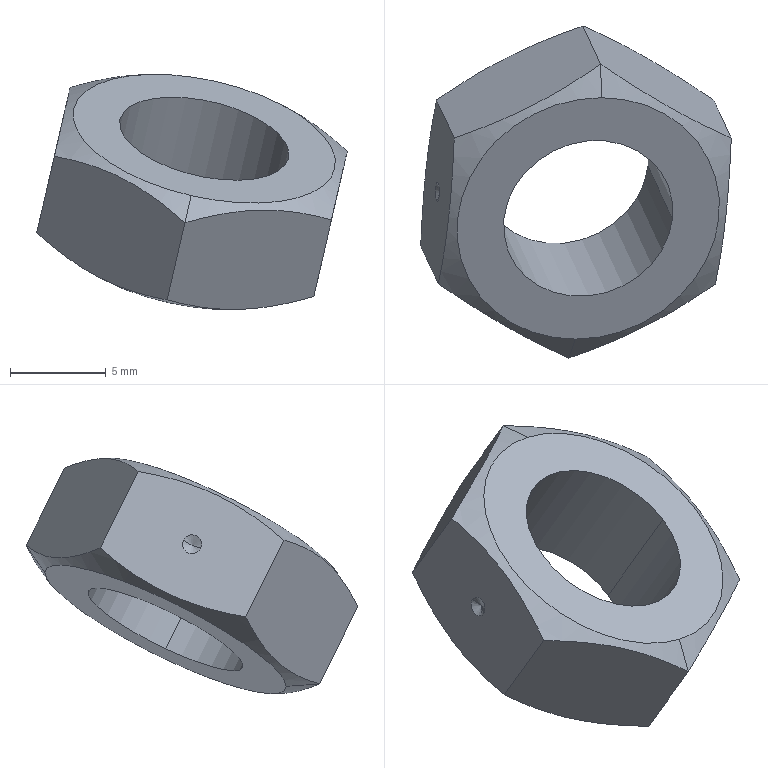Part | SolidWorks | features BaseBody 1 | 1 solid | 18 faces | box 16.219 x 17.338 x 12.294 mm | volume 776.179 mm3 | plane 8 | cone 8 | cylinder 2 | commonest cylinder face diameters 9.035 x2
STEP:
#1=CARTESIAN_POINT('',(1929.341,-170.963,831.295));
#2=VERTEX_POINT('',#1);
#3=CARTESIAN_POINT('',(1930.707,-158.364,837.245));
#4=VERTEX_POINT('',#3);
#5=CARTESIAN_POINT('',(1930.024,-164.664,834.27));
#6=DIRECTION('',(0.2015,-0.436,0.8771));
#7=DIRECTION('',(-0.09761,-0.8999,-0.425));
#8=AXIS2_PLACEMENT_3D('',#5,#6,#7);
#9=CIRCLE('',#8,7.);
#10=EDGE_CURVE('',#2,#4,#9,.T.);
#11=ORIENTED_EDGE('',*,*,#10,.T.);
#12=CARTESIAN_POINT('',(1930.024,-164.664,834.27));
#13=DIRECTION('',(0.2015,-0.436,0.8771));
#14=DIRECTION('',(0.09761,0.8999,0.425));
#15=AXIS2_PLACEMENT_3D('',#12,#13,#14);
#16=CIRCLE('',#15,7.);
#17=EDGE_CURVE('',#4,#2,#16,.T.);
#18=ORIENTED_EDGE('',*,*,#17,.T.);
#19=EDGE_LOOP('',(#11,#18));
#20=FACE_OUTER_BOUND('',#19,.T.);
#21=CARTESIAN_POINT('',(1934.427,-164.664,833.259));
#22=VERTEX_POINT('',#21);
#23=CARTESIAN_POINT('',(1925.621,-164.664,835.281));
#24=VERTEX_POINT('',#23);
#25=CARTESIAN_POINT('',(1930.024,-164.664,834.27));
#26=DIRECTION('',(-0.2015,0.436,-0.8771));
#27=DIRECTION('',(0.9746,0.,-0.2239));
#28=AXIS2_PLACEMENT_3D('',#25,#26,#27);
#29=CIRCLE('',#28,4.517);
#30=EDGE_CURVE('',#22,#24,#29,.T.);
#31=ORIENTED_EDGE('',*,*,#30,.T.);
#32=CARTESIAN_POINT('',(1930.024,-164.664,834.27));
#33=DIRECTION('',(-0.2015,0.436,-0.8771));
#34=DIRECTION('',(-0.9746,0.,0.2239));
#35=AXIS2_PLACEMENT_3D('',#32,#33,#34);
#36=CIRCLE('',#35,4.517);
#37=EDGE_CURVE('',#24,#22,#36,.T.);
#38=ORIENTED_EDGE('',*,*,#37,.T.);
#39=EDGE_LOOP('',(#31,#38));
#40=FACE_BOUND('',#39,.T.);
#41=CARTESIAN_POINT('',(1936.408,-171.215,829.546));
#42=DIRECTION('',(0.2015,-0.436,0.8771));
#43=DIRECTION('',(0.09761,0.8999,0.425));
#44=AXIS2_PLACEMENT_3D('',#41,#42,#43);
#45=PLANE('',#44);
#46=ADVANCED_FACE('',(#20,#40),#45,.T.);
#47=CARTESIAN_POINT('',(1924.342,-161.895,829.712));
#48=VERTEX_POINT('',#47);
#49=CARTESIAN_POINT('',(1925.621,-164.664,835.281));
#50=DIRECTION('',(-0.2015,0.436,-0.8771));
#51=VECTOR('',#50,1000.);
#52=LINE('',#49,#51);
#53=EDGE_CURVE('',#24,#48,#52,.T.);
#54=ORIENTED_EDGE('',*,*,#53,.T.);
#55=CARTESIAN_POINT('',(1933.147,-161.895,827.689));
#56=VERTEX_POINT('',#55);
#57=CARTESIAN_POINT('',(1928.744,-161.895,828.7));
#58=DIRECTION('',(-0.2015,0.436,-0.8771));
#59=DIRECTION('',(-0.9746,0.,0.2239));
#60=AXIS2_PLACEMENT_3D('',#57,#58,#59);
#61=CIRCLE('',#60,4.517);
#62=EDGE_CURVE('',#48,#56,#61,.T.);
#63=ORIENTED_EDGE('',*,*,#62,.T.);
#64=CARTESIAN_POINT('',(1934.427,-164.664,833.259));
#65=DIRECTION('',(0.2015,-0.436,0.8771));
#66=VECTOR('',#65,1000.);
#67=LINE('',#64,#66);
#68=EDGE_CURVE('',#56,#22,#67,.T.);
#69=ORIENTED_EDGE('',*,*,#68,.T.);
#70=ORIENTED_EDGE('',*,*,#37,.F.);
#71=EDGE_LOOP('',(#54,#63,#69,#70));
#72=FACE_OUTER_BOUND('',#71,.T.);
#73=CARTESIAN_POINT('',(1930.049,-164.719,834.381));
#74=DIRECTION('',(-0.2015,0.436,-0.8771));
#75=DIRECTION('',(-0.9746,0.,0.2239));
#76=AXIS2_PLACEMENT_3D('',#73,#74,#75);
#77=CYLINDRICAL_SURFACE('',#76,4.518);
#78=ADVANCED_FACE('',(#72),#77,.F.);
#79=ORIENTED_EDGE('',*,*,#68,.F.);
#80=CARTESIAN_POINT('',(1928.744,-161.895,828.7));
#81=DIRECTION('',(-0.2015,0.436,-0.8771));
#82=DIRECTION('',(0.9746,0.,-0.2239));
#83=AXIS2_PLACEMENT_3D('',#80,#81,#82);
#84=CIRCLE('',#83,4.517);
#85=EDGE_CURVE('',#56,#48,#84,.T.);
#86=ORIENTED_EDGE('',*,*,#85,.T.);
#87=ORIENTED_EDGE('',*,*,#53,.F.);
#88=ORIENTED_EDGE('',*,*,#30,.F.);
#89=EDGE_LOOP('',(#79,#86,#87,#88));
#90=FACE_OUTER_BOUND('',#89,.T.);
#91=CARTESIAN_POINT('',(1930.049,-164.719,834.381));
#92=DIRECTION('',(-0.2015,0.436,-0.8771));
#93=DIRECTION('',(-0.9746,0.,0.2239));
#94=AXIS2_PLACEMENT_3D('',#91,#92,#93);
#95=CYLINDRICAL_SURFACE('',#94,4.518);
#96=ADVANCED_FACE('',(#90),#95,.F.);
#97=CARTESIAN_POINT('',(1928.061,-168.194,825.726));
#98=VERTEX_POINT('',#97);
#99=CARTESIAN_POINT('',(1929.428,-155.595,831.675));
#100=VERTEX_POINT('',#99);
#101=CARTESIAN_POINT('',(1928.744,-161.895,828.7));
#102=DIRECTION('',(0.2015,-0.436,0.8771));
#103=DIRECTION('',(-0.09761,-0.8999,-0.425));
#104=AXIS2_PLACEMENT_3D('',#101,#102,#103);
#105=CIRCLE('',#104,7.);
#106=EDGE_CURVE('',#98,#100,#105,.T.);
#107=ORIENTED_EDGE('',*,*,#106,.F.);
#108=CARTESIAN_POINT('',(1928.744,-161.895,828.7));
#109=DIRECTION('',(0.2015,-0.436,0.8771));
#110=DIRECTION('',(0.09761,0.8999,0.425));
#111=AXIS2_PLACEMENT_3D('',#108,#109,#110);
#112=CIRCLE('',#111,7.);
#113=EDGE_CURVE('',#100,#98,#112,.T.);
#114=ORIENTED_EDGE('',*,*,#113,.F.);
#115=EDGE_LOOP('',(#107,#114));
#116=FACE_OUTER_BOUND('',#115,.T.);
#117=ORIENTED_EDGE('',*,*,#85,.F.);
#118=ORIENTED_EDGE('',*,*,#62,.F.);
#119=EDGE_LOOP('',(#117,#118));
#120=FACE_BOUND('',#119,.T.);
#121=CARTESIAN_POINT('',(1935.129,-168.446,823.977));
#122=DIRECTION('',(-0.2015,0.436,-0.8771));
#123=DIRECTION('',(-0.9746,0.,0.2239));
#124=AXIS2_PLACEMENT_3D('',#121,#122,#123);
#125=PLANE('',#124);
#126=ADVANCED_FACE('',(#116,#120),#125,.T.);
#127=CARTESIAN_POINT('',(1928.09,-169.945,825.849));
#128=VERTEX_POINT('',#127);
#129=CARTESIAN_POINT('',(1928.09,-169.945,825.849));
#130=DIRECTION('',(0.0162,-0.9974,0.07053));
#131=VECTOR('',#130,1000.);
#132=LINE('',#129,#131);
#133=EDGE_CURVE('',#98,#128,#132,.T.);
#134=ORIENTED_EDGE('',*,*,#133,.T.);
#135=CARTESIAN_POINT('',(1921.275,-166.094,829.347));
#136=VERTEX_POINT('',#135);
#137=CARTESIAN_POINT('',(1921.275,-166.094,829.347));
#138=CARTESIAN_POINT('',(1921.79,-166.32,828.884));
#139=CARTESIAN_POINT('',(1922.316,-166.563,828.45));
#140=CARTESIAN_POINT('',(1923.402,-167.102,827.665));
#141=CARTESIAN_POINT('',(1923.961,-167.397,827.315));
#142=CARTESIAN_POINT('',(1924.83,-167.888,826.868));
#143=CARTESIAN_POINT('',(1925.125,-168.06,826.732));
#144=CARTESIAN_POINT('',(1925.713,-168.411,826.49));
#145=CARTESIAN_POINT('',(1926.008,-168.593,826.383));
#146=CARTESIAN_POINT('',(1926.896,-169.151,826.098));
#147=CARTESIAN_POINT('',(1927.491,-169.541,825.957));
#148=CARTESIAN_POINT('',(1928.09,-169.945,825.849));
#149=B_SPLINE_CURVE_WITH_KNOTS('',3,(#137,#138,#139,#140,#141,#142,#143,#144,#145,#146,#147,#148),.UNSPECIFIED.,.F.,.F.,(4,2,2,2,2,4),(0.,0.002165,0.004331,0.005413,0.006496,0.008661),.UNSPECIFIED.);
#150=EDGE_CURVE('',#136,#128,#149,.T.);
#151=ORIENTED_EDGE('',*,*,#150,.F.);
#152=CARTESIAN_POINT('',(1922.101,-158.475,832.945));
#153=VERTEX_POINT('',#152);
#154=CARTESIAN_POINT('',(1922.101,-158.475,832.945));
#155=CARTESIAN_POINT('',(1921.994,-159.011,832.478));
#156=CARTESIAN_POINT('',(1921.893,-159.566,832.039));
#157=CARTESIAN_POINT('',(1921.71,-160.734,831.244));
#158=CARTESIAN_POINT('',(1921.629,-161.347,830.888));
#159=CARTESIAN_POINT('',(1921.523,-162.317,830.429));
#160=CARTESIAN_POINT('',(1921.491,-162.649,830.288));
#161=CARTESIAN_POINT('',(1921.433,-163.319,830.036));
#162=CARTESIAN_POINT('',(1921.407,-163.658,829.923));
#163=CARTESIAN_POINT('',(1921.338,-164.685,829.621));
#164=CARTESIAN_POINT('',(1921.302,-165.384,829.468));
#165=CARTESIAN_POINT('',(1921.275,-166.094,829.347));
#166=B_SPLINE_CURVE_WITH_KNOTS('',3,(#154,#155,#156,#157,#158,#159,#160,#161,#162,#163,#164,#165),.UNSPECIFIED.,.F.,.F.,(4,2,2,2,2,4),(0.,0.002137,0.004273,0.005342,0.00641,0.008546),.UNSPECIFIED.);
#167=EDGE_CURVE('',#153,#136,#166,.T.);
#168=ORIENTED_EDGE('',*,*,#167,.F.);
#169=CARTESIAN_POINT('',(1929.753,-154.61,833.091));
#170=VERTEX_POINT('',#169);
#171=CARTESIAN_POINT('',(1929.753,-154.61,833.091));
#172=CARTESIAN_POINT('',(1929.087,-154.837,832.9));
#173=CARTESIAN_POINT('',(1928.424,-155.082,832.741));
#174=CARTESIAN_POINT('',(1927.105,-155.623,832.514));
#175=CARTESIAN_POINT('',(1926.449,-155.92,832.446));
#176=CARTESIAN_POINT('',(1925.473,-156.413,832.427));
#177=CARTESIAN_POINT('',(1925.15,-156.585,832.434));
#178=CARTESIAN_POINT('',(1924.516,-156.938,832.475));
#179=CARTESIAN_POINT('',(1924.204,-157.12,832.509));
#180=CARTESIAN_POINT('',(1923.282,-157.679,832.644));
#181=CARTESIAN_POINT('',(1922.685,-158.071,832.779));
#182=CARTESIAN_POINT('',(1922.101,-158.475,832.945));
#183=B_SPLINE_CURVE_WITH_KNOTS('',3,(#171,#172,#173,#174,#175,#176,#177,#178,#179,#180,#181,#182),.UNSPECIFIED.,.F.,.F.,(4,2,2,2,2,4),(0.,0.002165,0.00433,0.005413,0.006496,0.008661),.UNSPECIFIED.);
#184=EDGE_CURVE('',#170,#153,#183,.T.);
#185=ORIENTED_EDGE('',*,*,#184,.F.);
#186=CARTESIAN_POINT('',(1929.753,-154.61,833.091));
#187=DIRECTION('',(-0.1853,-0.5614,-0.8066));
#188=VECTOR('',#187,1000.);
#189=LINE('',#186,#188);
#190=EDGE_CURVE('',#170,#100,#189,.T.);
#191=ORIENTED_EDGE('',*,*,#190,.T.);
#192=ORIENTED_EDGE('',*,*,#113,.T.);
#193=EDGE_LOOP('',(#134,#151,#168,#185,#191,#192));
#194=FACE_OUTER_BOUND('',#193,.T.);
#195=CARTESIAN_POINT('',(1928.741,-161.887,828.685));
#196=DIRECTION('',(0.2015,-0.436,0.8771));
#197=DIRECTION('',(-0.09761,-0.8999,-0.425));
#198=AXIS2_PLACEMENT_3D('',#195,#196,#197);
#199=CONICAL_SURFACE('',#198,6.969,1.047);
#200=ADVANCED_FACE('',(#194),#199,.T.);
#201=ORIENTED_EDGE('',*,*,#190,.F.);
#202=CARTESIAN_POINT('',(1936.574,-158.475,829.62));
#203=VERTEX_POINT('',#202);
#204=CARTESIAN_POINT('',(1936.574,-158.475,829.62));
#205=CARTESIAN_POINT('',(1935.977,-158.071,829.726));
#206=CARTESIAN_POINT('',(1935.382,-157.68,829.864));
#207=CARTESIAN_POINT('',(1934.202,-156.937,830.237));
#208=CARTESIAN_POINT('',(1933.617,-156.585,830.473));
#209=CARTESIAN_POINT('',(1932.746,-156.091,830.914));
#210=CARTESIAN_POINT('',(1932.458,-155.933,831.076));
#211=CARTESIAN_POINT('',(1931.894,-155.633,831.423));
#212=CARTESIAN_POINT('',(1931.617,-155.49,831.608));
#213=CARTESIAN_POINT('',(1930.798,-155.083,832.195));
#214=CARTESIAN_POINT('',(1930.27,-154.837,832.628));
#215=CARTESIAN_POINT('',(1929.753,-154.61,833.091));
#216=B_SPLINE_CURVE_WITH_KNOTS('',3,(#204,#205,#206,#207,#208,#209,#210,#211,#212,#213,#214,#215),.UNSPECIFIED.,.F.,.F.,(4,2,2,2,2,4),(0.,0.002165,0.004331,0.005413,0.006496,0.008661),.UNSPECIFIED.);
#217=EDGE_CURVE('',#203,#170,#216,.T.);
#218=ORIENTED_EDGE('',*,*,#217,.F.);
#219=CARTESIAN_POINT('',(1935.748,-166.094,826.023));
#220=VERTEX_POINT('',#219);
#221=CARTESIAN_POINT('',(1935.748,-166.094,826.023));
#222=CARTESIAN_POINT('',(1935.775,-165.385,826.143));
#223=CARTESIAN_POINT('',(1935.811,-164.688,826.296));
#224=CARTESIAN_POINT('',(1935.903,-163.324,826.697));
#225=CARTESIAN_POINT('',(1935.959,-162.657,826.944));
#226=CARTESIAN_POINT('',(1936.065,-161.686,827.402));
#227=CARTESIAN_POINT('',(1936.103,-161.367,827.569));
#228=CARTESIAN_POINT('',(1936.185,-160.749,827.925));
#229=CARTESIAN_POINT('',(1936.228,-160.449,828.114));
#230=CARTESIAN_POINT('',(1936.366,-159.569,828.713));
#231=CARTESIAN_POINT('',(1936.467,-159.011,829.152));
#232=CARTESIAN_POINT('',(1936.574,-158.475,829.62));
#233=B_SPLINE_CURVE_WITH_KNOTS('',3,(#221,#222,#223,#224,#225,#226,#227,#228,#229,#230,#231,#232),.UNSPECIFIED.,.F.,.F.,(4,2,2,2,2,4),(0.,0.002137,0.004273,0.005342,0.00641,0.008546),.UNSPECIFIED.);
#234=EDGE_CURVE('',#220,#203,#233,.T.);
#235=ORIENTED_EDGE('',*,*,#234,.F.);
#236=CARTESIAN_POINT('',(1928.09,-169.945,825.849));
#237=CARTESIAN_POINT('',(1928.674,-169.542,825.685));
#238=CARTESIAN_POINT('',(1929.27,-169.152,825.552));
#239=CARTESIAN_POINT('',(1930.497,-168.411,825.378));
#240=CARTESIAN_POINT('',(1931.127,-168.059,825.336));
#241=CARTESIAN_POINT('',(1932.104,-167.568,825.358));
#242=CARTESIAN_POINT('',(1932.434,-167.41,825.38));
#243=CARTESIAN_POINT('',(1933.093,-167.112,825.448));
#244=CARTESIAN_POINT('',(1933.424,-166.97,825.495));
#245=CARTESIAN_POINT('',(1934.417,-166.564,825.669));
#246=CARTESIAN_POINT('',(1935.081,-166.32,825.831));
#247=CARTESIAN_POINT('',(1935.748,-166.094,826.023));
#248=B_SPLINE_CURVE_WITH_KNOTS('',3,(#236,#237,#238,#239,#240,#241,#242,#243,#244,#245,#246,#247),.UNSPECIFIED.,.F.,.F.,(4,2,2,2,2,4),(0.,0.002165,0.00433,0.005413,0.006496,0.008661),.UNSPECIFIED.);
#249=EDGE_CURVE('',#128,#220,#248,.T.);
#250=ORIENTED_EDGE('',*,*,#249,.F.);
#251=ORIENTED_EDGE('',*,*,#133,.F.);
#252=ORIENTED_EDGE('',*,*,#106,.T.);
#253=EDGE_LOOP('',(#201,#218,#235,#250,#251,#252));
#254=FACE_OUTER_BOUND('',#253,.T.);
#255=CARTESIAN_POINT('',(1928.741,-161.887,828.685));
#256=DIRECTION('',(0.2015,-0.436,0.8771));
#257=DIRECTION('',(-0.09761,-0.8999,-0.425));
#258=AXIS2_PLACEMENT_3D('',#255,#256,#257);
#259=CONICAL_SURFACE('',#258,6.969,1.047);
#260=ADVANCED_FACE('',(#254),#259,.T.);
#261=CARTESIAN_POINT('',(1936.667,-168.084,830.025));
#262=VERTEX_POINT('',#261);
#263=CARTESIAN_POINT('',(1936.667,-168.084,830.025));
#264=DIRECTION('',(-0.2015,0.436,-0.8771));
#265=VECTOR('',#264,1000.);
#266=LINE('',#263,#265);
#267=EDGE_CURVE('',#262,#220,#266,.T.);
#268=ORIENTED_EDGE('',*,*,#267,.F.);
#269=CARTESIAN_POINT('',(1929.015,-171.948,829.88));
#270=VERTEX_POINT('',#269);
#271=CARTESIAN_POINT('',(1929.015,-171.948,829.88));
#272=CARTESIAN_POINT('',(1929.681,-171.721,830.07));
#273=CARTESIAN_POINT('',(1930.344,-171.477,830.229));
#274=CARTESIAN_POINT('',(1931.663,-170.935,830.457));
#275=CARTESIAN_POINT('',(1932.319,-170.638,830.525));
#276=CARTESIAN_POINT('',(1933.295,-170.145,830.543));
#277=CARTESIAN_POINT('',(1933.619,-169.974,830.536));
#278=CARTESIAN_POINT('',(1934.253,-169.621,830.495));
#279=CARTESIAN_POINT('',(1934.564,-169.439,830.461));
#280=CARTESIAN_POINT('',(1935.486,-168.879,830.326));
#281=CARTESIAN_POINT('',(1936.083,-168.488,830.191));
#282=CARTESIAN_POINT('',(1936.667,-168.084,830.025));
#283=B_SPLINE_CURVE_WITH_KNOTS('',3,(#271,#272,#273,#274,#275,#276,#277,#278,#279,#280,#281,#282),.UNSPECIFIED.,.F.,.F.,(4,2,2,2,2,4),(0.,0.002165,0.00433,0.005413,0.006496,0.008661),.UNSPECIFIED.);
#284=EDGE_CURVE('',#270,#262,#283,.T.);
#285=ORIENTED_EDGE('',*,*,#284,.F.);
#286=CARTESIAN_POINT('',(1929.015,-171.948,829.88));
#287=DIRECTION('',(-0.2015,0.436,-0.8771));
#288=VECTOR('',#287,1000.);
#289=LINE('',#286,#288);
#290=EDGE_CURVE('',#270,#128,#289,.T.);
#291=ORIENTED_EDGE('',*,*,#290,.T.);
#292=ORIENTED_EDGE('',*,*,#249,.T.);
#293=EDGE_LOOP('',(#268,#285,#291,#292));
#294=FACE_OUTER_BOUND('',#293,.T.);
#295=CARTESIAN_POINT('',(1936.98,-168.352,830.724));
#296=DIRECTION('',(0.4028,-0.7794,-0.48));
#297=DIRECTION('',(-0.8929,-0.45,-0.0186));
#298=AXIS2_PLACEMENT_3D('',#295,#296,#297);
#299=PLANE('',#298);
#300=ADVANCED_FACE('',(#294),#299,.T.);
#301=ORIENTED_EDGE('',*,*,#290,.F.);
#302=CARTESIAN_POINT('',(1922.194,-168.084,833.35));
#303=VERTEX_POINT('',#302);
#304=CARTESIAN_POINT('',(1922.194,-168.084,833.35));
#305=CARTESIAN_POINT('',(1922.791,-168.487,833.244));
#306=CARTESIAN_POINT('',(1923.386,-168.878,833.106));
#307=CARTESIAN_POINT('',(1924.566,-169.621,832.733));
#308=CARTESIAN_POINT('',(1925.152,-169.974,832.498));
#309=CARTESIAN_POINT('',(1926.022,-170.467,832.056));
#310=CARTESIAN_POINT('',(1926.31,-170.626,831.894));
#311=CARTESIAN_POINT('',(1926.875,-170.926,831.548));
#312=CARTESIAN_POINT('',(1927.152,-171.068,831.362));
#313=CARTESIAN_POINT('',(1927.97,-171.476,830.775));
#314=CARTESIAN_POINT('',(1928.499,-171.721,830.342));
#315=CARTESIAN_POINT('',(1929.015,-171.948,829.88));
#316=B_SPLINE_CURVE_WITH_KNOTS('',3,(#304,#305,#306,#307,#308,#309,#310,#311,#312,#313,#314,#315),.UNSPECIFIED.,.F.,.F.,(4,2,2,2,2,4),(0.,0.002165,0.004331,0.005413,0.006496,0.008661),.UNSPECIFIED.);
#317=EDGE_CURVE('',#303,#270,#316,.T.);
#318=ORIENTED_EDGE('',*,*,#317,.F.);
#319=CARTESIAN_POINT('',(1922.194,-168.084,833.35));
#320=DIRECTION('',(-0.2015,0.436,-0.8771));
#321=VECTOR('',#320,1000.);
#322=LINE('',#319,#321);
#323=EDGE_CURVE('',#303,#136,#322,.T.);
#324=ORIENTED_EDGE('',*,*,#323,.T.);
#325=ORIENTED_EDGE('',*,*,#150,.T.);
#326=EDGE_LOOP('',(#301,#318,#324,#325));
#327=FACE_OUTER_BOUND('',#326,.T.);
#328=CARTESIAN_POINT('',(1929.308,-172.364,830.492));
#329=DIRECTION('',(-0.5718,-0.7794,-0.2561));
#330=DIRECTION('',(-0.7952,0.45,0.4064));
#331=AXIS2_PLACEMENT_3D('',#328,#329,#330);
#332=PLANE('',#331);
#333=ADVANCED_FACE('',(#327),#332,.T.);
#334=ORIENTED_EDGE('',*,*,#323,.F.);
#335=CARTESIAN_POINT('',(1923.02,-160.465,836.948));
#336=VERTEX_POINT('',#335);
#337=CARTESIAN_POINT('',(1923.02,-160.465,836.948));
#338=CARTESIAN_POINT('',(1922.993,-161.173,836.827));
#339=CARTESIAN_POINT('',(1922.958,-161.871,836.674));
#340=CARTESIAN_POINT('',(1922.866,-163.235,836.274));
#341=CARTESIAN_POINT('',(1922.809,-163.901,836.026));
#342=CARTESIAN_POINT('',(1922.704,-164.872,835.568));
#343=CARTESIAN_POINT('',(1922.665,-165.191,835.401));
#344=CARTESIAN_POINT('',(1922.584,-165.809,835.046));
#345=CARTESIAN_POINT('',(1922.54,-166.11,834.856));
#346=CARTESIAN_POINT('',(1922.403,-166.99,834.257));
#347=CARTESIAN_POINT('',(1922.302,-167.547,833.818));
#348=CARTESIAN_POINT('',(1922.194,-168.084,833.35));
#349=B_SPLINE_CURVE_WITH_KNOTS('',3,(#337,#338,#339,#340,#341,#342,#343,#344,#345,#346,#347,#348),.UNSPECIFIED.,.F.,.F.,(4,2,2,2,2,4),(0.,0.002137,0.004273,0.005342,0.00641,0.008546),.UNSPECIFIED.);
#350=EDGE_CURVE('',#336,#303,#349,.T.);
#351=ORIENTED_EDGE('',*,*,#350,.F.);
#352=CARTESIAN_POINT('',(1923.02,-160.465,836.948));
#353=DIRECTION('',(-0.2015,0.436,-0.8771));
#354=VECTOR('',#353,1000.);
#355=LINE('',#352,#354);
#356=EDGE_CURVE('',#336,#153,#355,.T.);
#357=ORIENTED_EDGE('',*,*,#356,.T.);
#358=ORIENTED_EDGE('',*,*,#167,.T.);
#359=EDGE_LOOP('',(#334,#351,#357,#358));
#360=FACE_OUTER_BOUND('',#359,.T.);
#361=CARTESIAN_POINT('',(1922.196,-162.829,833.36));
#362=VERTEX_POINT('',#361);
#363=CARTESIAN_POINT('',(1922.099,-163.729,832.935));
#364=VERTEX_POINT('',#363);
#365=CARTESIAN_POINT('',(1922.148,-163.279,833.147));
#366=DIRECTION('',(-0.9746,0.,0.2239));
#367=DIRECTION('',(0.09761,0.8999,0.425));
#368=AXIS2_PLACEMENT_3D('',#365,#366,#367);
#369=CIRCLE('',#368,0.5);
#370=EDGE_CURVE('',#362,#364,#369,.T.);
#371=ORIENTED_EDGE('',*,*,#370,.F.);
#372=CARTESIAN_POINT('',(1922.148,-163.279,833.147));
#373=DIRECTION('',(-0.9746,0.,0.2239));
#374=DIRECTION('',(-0.09761,-0.8999,-0.425));
#375=AXIS2_PLACEMENT_3D('',#372,#373,#374);
#376=CIRCLE('',#375,0.5);
#377=EDGE_CURVE('',#364,#362,#376,.T.);
#378=ORIENTED_EDGE('',*,*,#377,.F.);
#379=EDGE_LOOP('',(#371,#378));
#380=FACE_BOUND('',#379,.T.);
#381=CARTESIAN_POINT('',(1922.332,-168.57,833.949));
#382=DIRECTION('',(-0.9746,0.,0.2239));
#383=DIRECTION('',(0.09761,0.8999,0.425));
#384=AXIS2_PLACEMENT_3D('',#381,#382,#383);
#385=PLANE('',#384);
#386=ADVANCED_FACE('',(#360,#380),#385,.T.);
#387=ORIENTED_EDGE('',*,*,#356,.F.);
#388=CARTESIAN_POINT('',(1930.679,-156.613,837.121));
#389=VERTEX_POINT('',#388);
#390=CARTESIAN_POINT('',(1930.679,-156.613,837.121));
#391=CARTESIAN_POINT('',(1930.094,-157.017,837.285));
#392=CARTESIAN_POINT('',(1929.498,-157.406,837.418));
#393=CARTESIAN_POINT('',(1928.272,-158.148,837.592));
#394=CARTESIAN_POINT('',(1927.641,-158.499,837.634));
#395=CARTESIAN_POINT('',(1926.664,-158.991,837.612));
#396=CARTESIAN_POINT('',(1926.334,-159.148,837.591));
#397=CARTESIAN_POINT('',(1925.675,-159.447,837.522));
#398=CARTESIAN_POINT('',(1925.345,-159.589,837.476));
#399=CARTESIAN_POINT('',(1924.352,-159.994,837.301));
#400=CARTESIAN_POINT('',(1923.687,-160.238,837.14));
#401=CARTESIAN_POINT('',(1923.02,-160.465,836.948));
#402=B_SPLINE_CURVE_WITH_KNOTS('',3,(#390,#391,#392,#393,#394,#395,#396,#397,#398,#399,#400,#401),.UNSPECIFIED.,.F.,.F.,(4,2,2,2,2,4),(0.,0.002165,0.00433,0.005413,0.006496,0.008661),.UNSPECIFIED.);
#403=EDGE_CURVE('',#389,#336,#402,.T.);
#404=ORIENTED_EDGE('',*,*,#403,.F.);
#405=CARTESIAN_POINT('',(1930.679,-156.613,837.121));
#406=DIRECTION('',(-0.2015,0.436,-0.8771));
#407=VECTOR('',#406,1000.);
#408=LINE('',#405,#407);
#409=EDGE_CURVE('',#389,#170,#408,.T.);
#410=ORIENTED_EDGE('',*,*,#409,.T.);
#411=ORIENTED_EDGE('',*,*,#184,.T.);
#412=EDGE_LOOP('',(#387,#404,#410,#411));
#413=FACE_OUTER_BOUND('',#412,.T.);
#414=CARTESIAN_POINT('',(1923.027,-160.887,837.64));
#415=DIRECTION('',(-0.4028,0.7794,0.48));
#416=DIRECTION('',(0.8929,0.45,0.0186));
#417=AXIS2_PLACEMENT_3D('',#414,#415,#416);
#418=PLANE('',#417);
#419=ADVANCED_FACE('',(#413),#418,.T.);
#420=ORIENTED_EDGE('',*,*,#409,.F.);
#421=CARTESIAN_POINT('',(1937.494,-160.465,833.623));
#422=VERTEX_POINT('',#421);
#423=CARTESIAN_POINT('',(1937.494,-160.465,833.623));
#424=CARTESIAN_POINT('',(1936.978,-160.239,834.086));
#425=CARTESIAN_POINT('',(1936.452,-159.995,834.52));
#426=CARTESIAN_POINT('',(1935.366,-159.456,835.305));
#427=CARTESIAN_POINT('',(1934.807,-159.161,835.655));
#428=CARTESIAN_POINT('',(1933.938,-158.67,836.102));
#429=CARTESIAN_POINT('',(1933.644,-158.499,836.238));
#430=CARTESIAN_POINT('',(1933.055,-158.147,836.48));
#431=CARTESIAN_POINT('',(1932.76,-157.966,836.588));
#432=CARTESIAN_POINT('',(1931.872,-157.408,836.872));
#433=CARTESIAN_POINT('',(1931.277,-157.017,837.013));
#434=CARTESIAN_POINT('',(1930.679,-156.613,837.121));
#435=B_SPLINE_CURVE_WITH_KNOTS('',3,(#423,#424,#425,#426,#427,#428,#429,#430,#431,#432,#433,#434),.UNSPECIFIED.,.F.,.F.,(4,2,2,2,2,4),(0.,0.002165,0.004331,0.005413,0.006496,0.008661),.UNSPECIFIED.);
#436=EDGE_CURVE('',#422,#389,#435,.T.);
#437=ORIENTED_EDGE('',*,*,#436,.F.);
#438=CARTESIAN_POINT('',(1937.494,-160.465,833.623));
#439=DIRECTION('',(-0.2015,0.436,-0.8771));
#440=VECTOR('',#439,1000.);
#441=LINE('',#438,#440);
#442=EDGE_CURVE('',#422,#203,#441,.T.);
#443=ORIENTED_EDGE('',*,*,#442,.T.);
#444=ORIENTED_EDGE('',*,*,#217,.T.);
#445=EDGE_LOOP('',(#420,#437,#443,#444));
#446=FACE_OUTER_BOUND('',#445,.T.);
#447=CARTESIAN_POINT('',(1930.699,-156.875,837.872));
#448=DIRECTION('',(0.5718,0.7794,0.2561));
#449=DIRECTION('',(0.7952,-0.45,-0.4064));
#450=AXIS2_PLACEMENT_3D('',#447,#448,#449);
#451=PLANE('',#450);
#452=ADVANCED_FACE('',(#446),#451,.T.);
#453=ORIENTED_EDGE('',*,*,#442,.F.);
#454=CARTESIAN_POINT('',(1936.667,-168.084,830.025));
#455=CARTESIAN_POINT('',(1936.775,-167.548,830.493));
#456=CARTESIAN_POINT('',(1936.875,-166.992,830.931));
#457=CARTESIAN_POINT('',(1937.058,-165.824,831.726));
#458=CARTESIAN_POINT('',(1937.14,-165.212,832.083));
#459=CARTESIAN_POINT('',(1937.245,-164.241,832.542));
#460=CARTESIAN_POINT('',(1937.277,-163.909,832.682));
#461=CARTESIAN_POINT('',(1937.335,-163.24,832.934));
#462=CARTESIAN_POINT('',(1937.361,-162.901,833.047));
#463=CARTESIAN_POINT('',(1937.431,-161.873,833.349));
#464=CARTESIAN_POINT('',(1937.466,-161.174,833.503));
#465=CARTESIAN_POINT('',(1937.494,-160.465,833.623));
#466=B_SPLINE_CURVE_WITH_KNOTS('',3,(#454,#455,#456,#457,#458,#459,#460,#461,#462,#463,#464,#465),.UNSPECIFIED.,.F.,.F.,(4,2,2,2,2,4),(0.,0.002137,0.004273,0.005342,0.00641,0.008546),.UNSPECIFIED.);
#467=EDGE_CURVE('',#262,#422,#466,.T.);
#468=ORIENTED_EDGE('',*,*,#467,.F.);
#469=ORIENTED_EDGE('',*,*,#267,.T.);
#470=ORIENTED_EDGE('',*,*,#234,.T.);
#471=EDGE_LOOP('',(#453,#468,#469,#470));
#472=FACE_OUTER_BOUND('',#471,.T.);
#473=CARTESIAN_POINT('',(1936.669,-162.829,830.035));
#474=VERTEX_POINT('',#473);
#475=CARTESIAN_POINT('',(1936.572,-163.729,829.61));
#476=VERTEX_POINT('',#475);
#477=CARTESIAN_POINT('',(1936.621,-163.279,829.823));
#478=DIRECTION('',(-0.9746,0.,0.2239));
#479=DIRECTION('',(0.09761,0.8999,0.425));
#480=AXIS2_PLACEMENT_3D('',#477,#478,#479);
#481=CIRCLE('',#480,0.5);
#482=EDGE_CURVE('',#474,#476,#481,.T.);
#483=ORIENTED_EDGE('',*,*,#482,.T.);
#484=CARTESIAN_POINT('',(1936.621,-163.279,829.823));
#485=DIRECTION('',(-0.9746,0.,0.2239));
#486=DIRECTION('',(-0.09761,-0.8999,-0.425));
#487=AXIS2_PLACEMENT_3D('',#484,#485,#486);
#488=CIRCLE('',#487,0.5);
#489=EDGE_CURVE('',#476,#474,#488,.T.);
#490=ORIENTED_EDGE('',*,*,#489,.T.);
#491=EDGE_LOOP('',(#483,#490));
#492=FACE_BOUND('',#491,.T.);
#493=CARTESIAN_POINT('',(1937.664,-160.646,834.366));
#494=DIRECTION('',(0.9746,0.,-0.2239));
#495=DIRECTION('',(-0.09761,-0.8999,-0.425));
#496=AXIS2_PLACEMENT_3D('',#493,#494,#495);
#497=PLANE('',#496);
#498=ADVANCED_FACE('',(#472,#492),#497,.T.);
#499=CARTESIAN_POINT('',(1929.341,-170.963,831.295));
#500=DIRECTION('',(0.1853,0.5614,0.8066));
#501=VECTOR('',#500,1000.);
#502=LINE('',#499,#501);
#503=EDGE_CURVE('',#270,#2,#502,.T.);
#504=ORIENTED_EDGE('',*,*,#503,.F.);
#505=ORIENTED_EDGE('',*,*,#284,.T.);
#506=ORIENTED_EDGE('',*,*,#467,.T.);
#507=ORIENTED_EDGE('',*,*,#436,.T.);
#508=CARTESIAN_POINT('',(1930.707,-158.364,837.245));
#509=DIRECTION('',(-0.0162,0.9974,-0.07053));
#510=VECTOR('',#509,1000.);
#511=LINE('',#508,#510);
#512=EDGE_CURVE('',#4,#389,#511,.T.);
#513=ORIENTED_EDGE('',*,*,#512,.F.);
#514=ORIENTED_EDGE('',*,*,#10,.F.);
#515=EDGE_LOOP('',(#504,#505,#506,#507,#513,#514));
#516=FACE_OUTER_BOUND('',#515,.T.);
#517=CARTESIAN_POINT('',(1929.84,-164.266,833.471));
#518=DIRECTION('',(-0.2015,0.436,-0.8771));
#519=DIRECTION('',(0.09761,0.8999,0.425));
#520=AXIS2_PLACEMENT_3D('',#517,#518,#519);
#521=CONICAL_SURFACE('',#520,8.578,1.047);
#522=ADVANCED_FACE('',(#516),#521,.T.);
#523=ORIENTED_EDGE('',*,*,#512,.T.);
#524=ORIENTED_EDGE('',*,*,#403,.T.);
#525=ORIENTED_EDGE('',*,*,#350,.T.);
#526=ORIENTED_EDGE('',*,*,#317,.T.);
#527=ORIENTED_EDGE('',*,*,#503,.T.);
#528=ORIENTED_EDGE('',*,*,#17,.F.);
#529=EDGE_LOOP('',(#523,#524,#525,#526,#527,#528));
#530=FACE_OUTER_BOUND('',#529,.T.);
#531=CARTESIAN_POINT('',(1929.84,-164.266,833.471));
#532=DIRECTION('',(-0.2015,0.436,-0.8771));
#533=DIRECTION('',(0.09761,0.8999,0.425));
#534=AXIS2_PLACEMENT_3D('',#531,#532,#533);
#535=CONICAL_SURFACE('',#534,8.578,1.047);
#536=ADVANCED_FACE('',(#530),#535,.T.);
#537=CARTESIAN_POINT('',(1936.339,-163.279,829.887));
#538=VERTEX_POINT('',#537);
#539=CARTESIAN_POINT('',(1936.339,-163.279,829.887));
#540=DIRECTION('',(0.4028,-0.7794,-0.48));
#541=VECTOR('',#540,1000.);
#542=LINE('',#539,#541);
#543=EDGE_CURVE('',#538,#476,#542,.T.);
#544=ORIENTED_EDGE('',*,*,#543,.F.);
#545=CARTESIAN_POINT('',(1936.339,-163.279,829.887));
#546=DIRECTION('',(-0.5718,-0.7794,-0.2561));
#547=VECTOR('',#546,1000.);
#548=LINE('',#545,#547);
#549=EDGE_CURVE('',#474,#538,#548,.T.);
#550=ORIENTED_EDGE('',*,*,#549,.F.);
#551=ORIENTED_EDGE('',*,*,#489,.F.);
#552=EDGE_LOOP('',(#544,#550,#551));
#553=FACE_OUTER_BOUND('',#552,.T.);
#554=CARTESIAN_POINT('',(1936.635,-163.279,829.819));
#555=DIRECTION('',(0.9746,0.,-0.2239));
#556=DIRECTION('',(-0.09761,-0.8999,-0.425));
#557=AXIS2_PLACEMENT_3D('',#554,#555,#556);
#558=CONICAL_SURFACE('',#557,0.526,1.047);
#559=ADVANCED_FACE('',(#553),#558,.F.);
#560=ORIENTED_EDGE('',*,*,#549,.T.);
#561=ORIENTED_EDGE('',*,*,#543,.T.);
#562=ORIENTED_EDGE('',*,*,#482,.F.);
#563=EDGE_LOOP('',(#560,#561,#562));
#564=FACE_OUTER_BOUND('',#563,.T.);
#565=CARTESIAN_POINT('',(1936.635,-163.279,829.819));
#566=DIRECTION('',(0.9746,0.,-0.2239));
#567=DIRECTION('',(-0.09761,-0.8999,-0.425));
#568=AXIS2_PLACEMENT_3D('',#565,#566,#567);
#569=CONICAL_SURFACE('',#568,0.526,1.047);
#570=ADVANCED_FACE('',(#564),#569,.F.);
#571=CARTESIAN_POINT('',(1922.429,-163.279,833.083));
#572=VERTEX_POINT('',#571);
#573=CARTESIAN_POINT('',(1922.429,-163.279,833.083));
#574=DIRECTION('',(-0.4028,0.7794,0.48));
#575=VECTOR('',#574,1000.);
#576=LINE('',#573,#575);
#577=EDGE_CURVE('',#572,#362,#576,.T.);
#578=ORIENTED_EDGE('',*,*,#577,.F.);
#579=CARTESIAN_POINT('',(1922.429,-163.279,833.083));
#580=DIRECTION('',(0.5718,0.7794,0.2561));
#581=VECTOR('',#580,1000.);
#582=LINE('',#579,#581);
#583=EDGE_CURVE('',#364,#572,#582,.T.);
#584=ORIENTED_EDGE('',*,*,#583,.F.);
#585=ORIENTED_EDGE('',*,*,#377,.T.);
#586=EDGE_LOOP('',(#578,#584,#585));
#587=FACE_OUTER_BOUND('',#586,.T.);
#588=CARTESIAN_POINT('',(947.809,-163.279,1056.951));
#589=DIRECTION('',(-0.9746,0.,0.2239));
#590=DIRECTION('',(0.09761,0.8999,0.425));
#591=AXIS2_PLACEMENT_3D('',#588,#589,#590);
#592=CONICAL_SURFACE('',#591,1732.051,1.047);
#593=ADVANCED_FACE('',(#587),#592,.F.);
#594=ORIENTED_EDGE('',*,*,#583,.T.);
#595=ORIENTED_EDGE('',*,*,#577,.T.);
#596=ORIENTED_EDGE('',*,*,#370,.T.);
#597=EDGE_LOOP('',(#594,#595,#596));
#598=FACE_OUTER_BOUND('',#597,.T.);
#599=CARTESIAN_POINT('',(947.809,-163.279,1056.951));
#600=DIRECTION('',(-0.9746,0.,0.2239));
#601=DIRECTION('',(0.09761,0.8999,0.425));
#602=AXIS2_PLACEMENT_3D('',#599,#600,#601);
#603=CONICAL_SURFACE('',#602,1732.051,1.047);
#604=ADVANCED_FACE('',(#598),#603,.F.);
#605=CLOSED_SHELL('',(#46,#78,#96,#126,#200,#260,#300,#333,#386,#419,#452,#498,#522,#536,#559,#570,#593,#604));
#606=MANIFOLD_SOLID_BREP('',#605);
#607=CARTESIAN_POINT('',(0.,0.,0.));
#608=DIRECTION('',(0.,0.,1.));
#609=DIRECTION('',(1.,0.,0.));
#610=AXIS2_PLACEMENT_3D('',#607,#608,#609);
#611=(LENGTH_UNIT()NAMED_UNIT(*)SI_UNIT(.MILLI.,.METRE.));
#612=UNCERTAINTY_MEASURE_WITH_UNIT(LENGTH_MEASURE(0.00001),#611,'','');
#613=(NAMED_UNIT(*)PLANE_ANGLE_UNIT()SI_UNIT($,.RADIAN.));
#614=(NAMED_UNIT(*)SI_UNIT($,.STERADIAN.)SOLID_ANGLE_UNIT());
#615=(GEOMETRIC_REPRESENTATION_CONTEXT(3)GLOBAL_UNCERTAINTY_ASSIGNED_CONTEXT((#612))GLOBAL_UNIT_ASSIGNED_CONTEXT((#611,#613,#614))REPRESENTATION_CONTEXT('',''));
#616=ADVANCED_BREP_SHAPE_REPRESENTATION('',(#606,#610),#615);